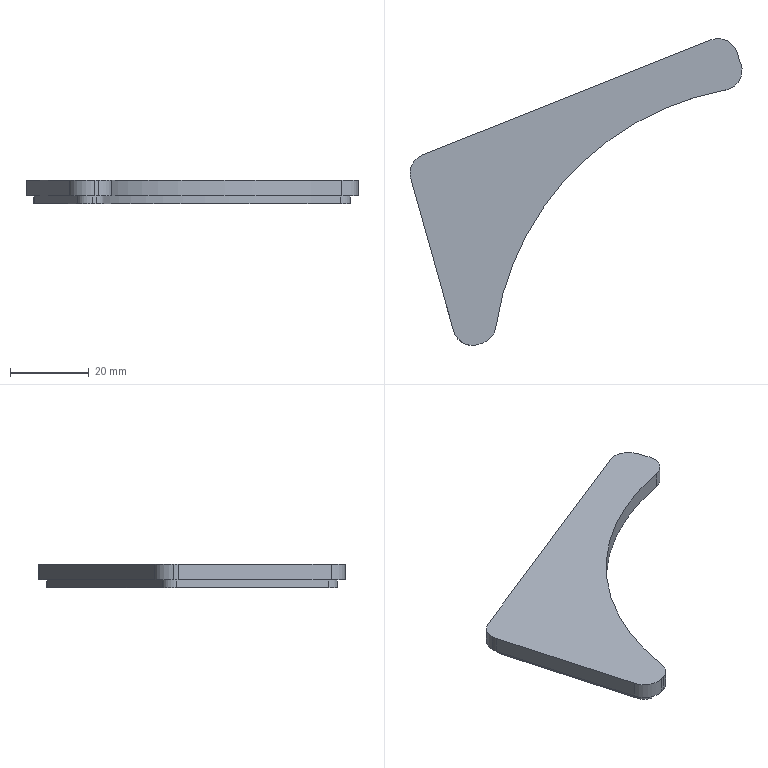Part | SolidWorks | features Extrusion 1, ICE 1 | 1 solid | 25 faces | box 84.083 x 77.703 x 6 mm | volume 11123 mm3 | cylinder 14 | plane 11 | commonest cylinder face diameters 6 x6 10 x6 144 x1 148 x1
STEP:
#1=CARTESIAN_POINT('',(135.377,149.372,4.));
#2=VERTEX_POINT('',#1);
#3=CARTESIAN_POINT('',(135.564,148.019,4.));
#4=VERTEX_POINT('',#3);
#5=CARTESIAN_POINT('',(140.377,149.372,4.));
#6=DIRECTION('',(0.,0.,1.));
#7=DIRECTION('',(-1.,0.,0.));
#8=AXIS2_PLACEMENT_3D('',#5,#6,#7);
#9=CIRCLE('',#8,5.);
#10=EDGE_CURVE('',#2,#4,#9,.T.);
#11=ORIENTED_EDGE('',*,*,#10,.F.);
#12=CARTESIAN_POINT('',(135.377,149.372,0.));
#13=VERTEX_POINT('',#12);
#14=CARTESIAN_POINT('',(135.377,149.372,4.));
#15=DIRECTION('',(0.,0.,-1.));
#16=VECTOR('',#15,1000.);
#17=LINE('',#14,#16);
#18=EDGE_CURVE('',#2,#13,#17,.T.);
#19=ORIENTED_EDGE('',*,*,#18,.T.);
#20=CARTESIAN_POINT('',(135.564,148.019,0.));
#21=VERTEX_POINT('',#20);
#22=CARTESIAN_POINT('',(140.377,149.372,0.));
#23=DIRECTION('',(0.,0.,1.));
#24=DIRECTION('',(-1.,0.,0.));
#25=AXIS2_PLACEMENT_3D('',#22,#23,#24);
#26=CIRCLE('',#25,5.);
#27=EDGE_CURVE('',#13,#21,#26,.T.);
#28=ORIENTED_EDGE('',*,*,#27,.T.);
#29=CARTESIAN_POINT('',(135.564,148.019,4.));
#30=DIRECTION('',(0.,0.,-1.));
#31=VECTOR('',#30,1000.);
#32=LINE('',#29,#31);
#33=EDGE_CURVE('',#4,#21,#32,.T.);
#34=ORIENTED_EDGE('',*,*,#33,.F.);
#35=EDGE_LOOP('',(#11,#19,#28,#34));
#36=FACE_OUTER_BOUND('',#35,.T.);
#37=CARTESIAN_POINT('',(140.377,149.372,4.));
#38=DIRECTION('',(0.,0.,-1.));
#39=DIRECTION('',(-1.,0.,0.));
#40=AXIS2_PLACEMENT_3D('',#37,#38,#39);
#41=CYLINDRICAL_SURFACE('',#40,5.);
#42=ADVANCED_FACE('',(#36),#41,.T.);
#43=CARTESIAN_POINT('',(214.999,172.437,-2.));
#44=VERTEX_POINT('',#43);
#45=CARTESIAN_POINT('',(217.46,175.388,-2.));
#46=VERTEX_POINT('',#45);
#47=CARTESIAN_POINT('',(214.46,175.388,-2.));
#48=DIRECTION('',(0.,0.,1.));
#49=DIRECTION('',(1.,0.,0.));
#50=AXIS2_PLACEMENT_3D('',#47,#48,#49);
#51=CIRCLE('',#50,3.);
#52=EDGE_CURVE('',#44,#46,#51,.T.);
#53=ORIENTED_EDGE('',*,*,#52,.T.);
#54=CARTESIAN_POINT('',(217.46,175.388,0.));
#55=VERTEX_POINT('',#54);
#56=CARTESIAN_POINT('',(217.46,175.388,-2.));
#57=DIRECTION('',(0.,0.,1.));
#58=VECTOR('',#57,1000.);
#59=LINE('',#56,#58);
#60=EDGE_CURVE('',#46,#55,#59,.T.);
#61=ORIENTED_EDGE('',*,*,#60,.T.);
#62=CARTESIAN_POINT('',(214.999,172.437,0.));
#63=VERTEX_POINT('',#62);
#64=CARTESIAN_POINT('',(214.46,175.388,0.));
#65=DIRECTION('',(0.,0.,1.));
#66=DIRECTION('',(1.,0.,0.));
#67=AXIS2_PLACEMENT_3D('',#64,#65,#66);
#68=CIRCLE('',#67,3.);
#69=EDGE_CURVE('',#63,#55,#68,.T.);
#70=ORIENTED_EDGE('',*,*,#69,.F.);
#71=CARTESIAN_POINT('',(214.999,172.437,-2.));
#72=DIRECTION('',(0.,0.,1.));
#73=VECTOR('',#72,1000.);
#74=LINE('',#71,#73);
#75=EDGE_CURVE('',#44,#63,#74,.T.);
#76=ORIENTED_EDGE('',*,*,#75,.F.);
#77=EDGE_LOOP('',(#53,#61,#70,#76));
#78=FACE_OUTER_BOUND('',#77,.T.);
#79=CARTESIAN_POINT('',(214.46,175.388,-2.));
#80=DIRECTION('',(0.,0.,1.));
#81=DIRECTION('',(1.,0.,0.));
#82=AXIS2_PLACEMENT_3D('',#79,#80,#81);
#83=CYLINDRICAL_SURFACE('',#82,3.);
#84=ADVANCED_FACE('',(#78),#83,.T.);
#85=CARTESIAN_POINT('',(139.266,152.159,0.));
#86=VERTEX_POINT('',#85);
#87=CARTESIAN_POINT('',(137.489,148.561,0.));
#88=VERTEX_POINT('',#87);
#89=CARTESIAN_POINT('',(140.377,149.372,0.));
#90=DIRECTION('',(0.,0.,1.));
#91=DIRECTION('',(1.,0.,0.));
#92=AXIS2_PLACEMENT_3D('',#89,#90,#91);
#93=CIRCLE('',#92,3.);
#94=EDGE_CURVE('',#86,#88,#93,.T.);
#95=ORIENTED_EDGE('',*,*,#94,.F.);
#96=CARTESIAN_POINT('',(139.266,152.159,-2.));
#97=VERTEX_POINT('',#96);
#98=CARTESIAN_POINT('',(139.266,152.159,-2.));
#99=DIRECTION('',(0.,0.,1.));
#100=VECTOR('',#99,1000.);
#101=LINE('',#98,#100);
#102=EDGE_CURVE('',#97,#86,#101,.T.);
#103=ORIENTED_EDGE('',*,*,#102,.F.);
#104=CARTESIAN_POINT('',(137.489,148.561,-2.));
#105=VERTEX_POINT('',#104);
#106=CARTESIAN_POINT('',(140.377,149.372,-2.));
#107=DIRECTION('',(0.,0.,1.));
#108=DIRECTION('',(1.,0.,0.));
#109=AXIS2_PLACEMENT_3D('',#106,#107,#108);
#110=CIRCLE('',#109,3.);
#111=EDGE_CURVE('',#97,#105,#110,.T.);
#112=ORIENTED_EDGE('',*,*,#111,.T.);
#113=CARTESIAN_POINT('',(137.489,148.561,-2.));
#114=DIRECTION('',(0.,0.,1.));
#115=VECTOR('',#114,1000.);
#116=LINE('',#113,#115);
#117=EDGE_CURVE('',#105,#88,#116,.T.);
#118=ORIENTED_EDGE('',*,*,#117,.T.);
#119=EDGE_LOOP('',(#95,#103,#112,#118));
#120=FACE_OUTER_BOUND('',#119,.T.);
#121=CARTESIAN_POINT('',(140.377,149.372,-2.));
#122=DIRECTION('',(0.,0.,1.));
#123=DIRECTION('',(1.,0.,0.));
#124=AXIS2_PLACEMENT_3D('',#121,#122,#123);
#125=CYLINDRICAL_SURFACE('',#124,3.);
#126=ADVANCED_FACE('',(#120),#125,.T.);
#127=CARTESIAN_POINT('',(212.285,181.276,0.));
#128=VERTEX_POINT('',#127);
#129=CARTESIAN_POINT('',(212.285,181.276,0.));
#130=DIRECTION('',(-0.9289,-0.3704,0.));
#131=VECTOR('',#130,1000.);
#132=LINE('',#129,#131);
#133=EDGE_CURVE('',#128,#86,#132,.T.);
#134=ORIENTED_EDGE('',*,*,#133,.F.);
#135=CARTESIAN_POINT('',(212.285,181.276,-2.));
#136=VERTEX_POINT('',#135);
#137=CARTESIAN_POINT('',(212.285,181.276,-2.));
#138=DIRECTION('',(0.,0.,1.));
#139=VECTOR('',#138,1000.);
#140=LINE('',#137,#139);
#141=EDGE_CURVE('',#136,#128,#140,.T.);
#142=ORIENTED_EDGE('',*,*,#141,.F.);
#143=CARTESIAN_POINT('',(212.285,181.276,-2.));
#144=DIRECTION('',(-0.9289,-0.3704,0.));
#145=VECTOR('',#144,1000.);
#146=LINE('',#143,#145);
#147=EDGE_CURVE('',#136,#97,#146,.T.);
#148=ORIENTED_EDGE('',*,*,#147,.T.);
#149=ORIENTED_EDGE('',*,*,#102,.T.);
#150=EDGE_LOOP('',(#134,#142,#148,#149));
#151=FACE_OUTER_BOUND('',#150,.T.);
#152=CARTESIAN_POINT('',(212.285,181.276,-2.));
#153=DIRECTION('',(-0.3704,0.9289,0.));
#154=DIRECTION('',(-0.9289,-0.3704,0.));
#155=AXIS2_PLACEMENT_3D('',#152,#153,#154);
#156=PLANE('',#155);
#157=ADVANCED_FACE('',(#151),#156,.T.);
#158=CARTESIAN_POINT('',(216.234,179.463,0.));
#159=VERTEX_POINT('',#158);
#160=CARTESIAN_POINT('',(213.396,178.489,0.));
#161=DIRECTION('',(0.,0.,1.));
#162=DIRECTION('',(1.,0.,0.));
#163=AXIS2_PLACEMENT_3D('',#160,#161,#162);
#164=CIRCLE('',#163,3.);
#165=EDGE_CURVE('',#159,#128,#164,.T.);
#166=ORIENTED_EDGE('',*,*,#165,.F.);
#167=CARTESIAN_POINT('',(216.234,179.463,-2.));
#168=VERTEX_POINT('',#167);
#169=CARTESIAN_POINT('',(216.234,179.463,-2.));
#170=DIRECTION('',(0.,0.,1.));
#171=VECTOR('',#170,1000.);
#172=LINE('',#169,#171);
#173=EDGE_CURVE('',#168,#159,#172,.T.);
#174=ORIENTED_EDGE('',*,*,#173,.F.);
#175=CARTESIAN_POINT('',(213.396,178.489,-2.));
#176=DIRECTION('',(0.,0.,1.));
#177=DIRECTION('',(1.,0.,0.));
#178=AXIS2_PLACEMENT_3D('',#175,#176,#177);
#179=CIRCLE('',#178,3.);
#180=EDGE_CURVE('',#168,#136,#179,.T.);
#181=ORIENTED_EDGE('',*,*,#180,.T.);
#182=ORIENTED_EDGE('',*,*,#141,.T.);
#183=EDGE_LOOP('',(#166,#174,#181,#182));
#184=FACE_OUTER_BOUND('',#183,.T.);
#185=CARTESIAN_POINT('',(213.396,178.489,-2.));
#186=DIRECTION('',(0.,0.,1.));
#187=DIRECTION('',(1.,0.,0.));
#188=AXIS2_PLACEMENT_3D('',#185,#186,#187);
#189=CYLINDRICAL_SURFACE('',#188,3.);
#190=ADVANCED_FACE('',(#184),#189,.T.);
#191=CARTESIAN_POINT('',(217.298,176.361,0.));
#192=VERTEX_POINT('',#191);
#193=CARTESIAN_POINT('',(217.298,176.361,0.));
#194=DIRECTION('',(-0.3245,0.9459,0.));
#195=VECTOR('',#194,1000.);
#196=LINE('',#193,#195);
#197=EDGE_CURVE('',#192,#159,#196,.T.);
#198=ORIENTED_EDGE('',*,*,#197,.F.);
#199=CARTESIAN_POINT('',(217.298,176.361,-2.));
#200=VERTEX_POINT('',#199);
#201=CARTESIAN_POINT('',(217.298,176.361,-2.));
#202=DIRECTION('',(0.,0.,1.));
#203=VECTOR('',#202,1000.);
#204=LINE('',#201,#203);
#205=EDGE_CURVE('',#200,#192,#204,.T.);
#206=ORIENTED_EDGE('',*,*,#205,.F.);
#207=CARTESIAN_POINT('',(217.298,176.361,-2.));
#208=DIRECTION('',(-0.3245,0.9459,0.));
#209=VECTOR('',#208,1000.);
#210=LINE('',#207,#209);
#211=EDGE_CURVE('',#200,#168,#210,.T.);
#212=ORIENTED_EDGE('',*,*,#211,.T.);
#213=ORIENTED_EDGE('',*,*,#173,.T.);
#214=EDGE_LOOP('',(#198,#206,#212,#213));
#215=FACE_OUTER_BOUND('',#214,.T.);
#216=CARTESIAN_POINT('',(217.298,176.361,-2.));
#217=DIRECTION('',(0.9459,0.3245,0.));
#218=DIRECTION('',(-0.3245,0.9459,0.));
#219=AXIS2_PLACEMENT_3D('',#216,#217,#218);
#220=PLANE('',#219);
#221=ADVANCED_FACE('',(#215),#220,.T.);
#222=ORIENTED_EDGE('',*,*,#60,.F.);
#223=CARTESIAN_POINT('',(214.46,175.388,-2.));
#224=DIRECTION('',(0.,0.,1.));
#225=DIRECTION('',(1.,0.,0.));
#226=AXIS2_PLACEMENT_3D('',#223,#224,#225);
#227=CIRCLE('',#226,3.);
#228=EDGE_CURVE('',#46,#200,#227,.T.);
#229=ORIENTED_EDGE('',*,*,#228,.T.);
#230=ORIENTED_EDGE('',*,*,#205,.T.);
#231=CARTESIAN_POINT('',(214.46,175.388,0.));
#232=DIRECTION('',(0.,0.,1.));
#233=DIRECTION('',(1.,0.,0.));
#234=AXIS2_PLACEMENT_3D('',#231,#232,#233);
#235=CIRCLE('',#234,3.);
#236=EDGE_CURVE('',#55,#192,#235,.T.);
#237=ORIENTED_EDGE('',*,*,#236,.F.);
#238=EDGE_LOOP('',(#222,#229,#230,#237));
#239=FACE_OUTER_BOUND('',#238,.T.);
#240=CARTESIAN_POINT('',(214.46,175.388,-2.));
#241=DIRECTION('',(0.,0.,1.));
#242=DIRECTION('',(1.,0.,0.));
#243=AXIS2_PLACEMENT_3D('',#240,#241,#242);
#244=CYLINDRICAL_SURFACE('',#243,3.);
#245=ADVANCED_FACE('',(#239),#244,.T.);
#246=CARTESIAN_POINT('',(155.118,110.657,0.));
#247=VERTEX_POINT('',#246);
#248=CARTESIAN_POINT('',(228.293,99.641,0.));
#249=DIRECTION('',(0.,0.,-1.));
#250=DIRECTION('',(1.,0.,0.));
#251=AXIS2_PLACEMENT_3D('',#248,#249,#250);
#252=CIRCLE('',#251,74.);
#253=EDGE_CURVE('',#247,#63,#252,.T.);
#254=ORIENTED_EDGE('',*,*,#253,.F.);
#255=CARTESIAN_POINT('',(155.118,110.657,-2.));
#256=VERTEX_POINT('',#255);
#257=CARTESIAN_POINT('',(155.118,110.657,-2.));
#258=DIRECTION('',(0.,0.,1.));
#259=VECTOR('',#258,1000.);
#260=LINE('',#257,#259);
#261=EDGE_CURVE('',#256,#247,#260,.T.);
#262=ORIENTED_EDGE('',*,*,#261,.F.);
#263=CARTESIAN_POINT('',(228.293,99.641,-2.));
#264=DIRECTION('',(0.,0.,-1.));
#265=DIRECTION('',(1.,0.,0.));
#266=AXIS2_PLACEMENT_3D('',#263,#264,#265);
#267=CIRCLE('',#266,74.);
#268=EDGE_CURVE('',#256,#44,#267,.T.);
#269=ORIENTED_EDGE('',*,*,#268,.T.);
#270=ORIENTED_EDGE('',*,*,#75,.T.);
#271=EDGE_LOOP('',(#254,#262,#269,#270));
#272=FACE_OUTER_BOUND('',#271,.T.);
#273=CARTESIAN_POINT('',(228.293,99.641,-2.));
#274=DIRECTION('',(0.,0.,1.));
#275=DIRECTION('',(1.,0.,0.));
#276=AXIS2_PLACEMENT_3D('',#273,#274,#275);
#277=CYLINDRICAL_SURFACE('',#276,74.);
#278=ADVANCED_FACE('',(#272),#277,.F.);
#279=CARTESIAN_POINT('',(153.125,108.266,0.));
#280=VERTEX_POINT('',#279);
#281=CARTESIAN_POINT('',(152.151,111.104,0.));
#282=DIRECTION('',(0.,0.,1.));
#283=DIRECTION('',(1.,0.,0.));
#284=AXIS2_PLACEMENT_3D('',#281,#282,#283);
#285=CIRCLE('',#284,3.);
#286=EDGE_CURVE('',#280,#247,#285,.T.);
#287=ORIENTED_EDGE('',*,*,#286,.F.);
#288=CARTESIAN_POINT('',(153.125,108.266,-2.));
#289=VERTEX_POINT('',#288);
#290=CARTESIAN_POINT('',(153.125,108.266,-2.));
#291=DIRECTION('',(0.,0.,1.));
#292=VECTOR('',#291,1000.);
#293=LINE('',#290,#292);
#294=EDGE_CURVE('',#289,#280,#293,.T.);
#295=ORIENTED_EDGE('',*,*,#294,.F.);
#296=CARTESIAN_POINT('',(152.151,111.104,-2.));
#297=DIRECTION('',(0.,0.,1.));
#298=DIRECTION('',(1.,0.,0.));
#299=AXIS2_PLACEMENT_3D('',#296,#297,#298);
#300=CIRCLE('',#299,3.);
#301=EDGE_CURVE('',#289,#256,#300,.T.);
#302=ORIENTED_EDGE('',*,*,#301,.T.);
#303=ORIENTED_EDGE('',*,*,#261,.T.);
#304=EDGE_LOOP('',(#287,#295,#302,#303));
#305=FACE_OUTER_BOUND('',#304,.T.);
#306=CARTESIAN_POINT('',(152.151,111.104,-2.));
#307=DIRECTION('',(0.,0.,1.));
#308=DIRECTION('',(1.,0.,0.));
#309=AXIS2_PLACEMENT_3D('',#306,#307,#308);
#310=CYLINDRICAL_SURFACE('',#309,3.);
#311=ADVANCED_FACE('',(#305),#310,.T.);
#312=CARTESIAN_POINT('',(152.197,107.948,0.));
#313=VERTEX_POINT('',#312);
#314=CARTESIAN_POINT('',(152.197,107.948,0.));
#315=DIRECTION('',(0.9459,0.3245,0.));
#316=VECTOR('',#315,1000.);
#317=LINE('',#314,#316);
#318=EDGE_CURVE('',#313,#280,#317,.T.);
#319=ORIENTED_EDGE('',*,*,#318,.F.);
#320=CARTESIAN_POINT('',(152.197,107.948,-2.));
#321=VERTEX_POINT('',#320);
#322=CARTESIAN_POINT('',(152.197,107.948,-2.));
#323=DIRECTION('',(0.,0.,1.));
#324=VECTOR('',#323,1000.);
#325=LINE('',#322,#324);
#326=EDGE_CURVE('',#321,#313,#325,.T.);
#327=ORIENTED_EDGE('',*,*,#326,.F.);
#328=CARTESIAN_POINT('',(152.197,107.948,-2.));
#329=DIRECTION('',(0.9459,0.3245,0.));
#330=VECTOR('',#329,1000.);
#331=LINE('',#328,#330);
#332=EDGE_CURVE('',#321,#289,#331,.T.);
#333=ORIENTED_EDGE('',*,*,#332,.T.);
#334=ORIENTED_EDGE('',*,*,#294,.T.);
#335=EDGE_LOOP('',(#319,#327,#333,#334));
#336=FACE_OUTER_BOUND('',#335,.T.);
#337=CARTESIAN_POINT('',(152.197,107.948,-2.));
#338=DIRECTION('',(0.3245,-0.9459,0.));
#339=DIRECTION('',(0.9459,0.3245,0.));
#340=AXIS2_PLACEMENT_3D('',#337,#338,#339);
#341=PLANE('',#340);
#342=ADVANCED_FACE('',(#336),#341,.T.);
#343=CARTESIAN_POINT('',(148.336,109.974,0.));
#344=VERTEX_POINT('',#343);
#345=CARTESIAN_POINT('',(151.224,110.786,0.));
#346=DIRECTION('',(0.,0.,1.));
#347=DIRECTION('',(1.,0.,0.));
#348=AXIS2_PLACEMENT_3D('',#345,#346,#347);
#349=CIRCLE('',#348,3.);
#350=EDGE_CURVE('',#344,#313,#349,.T.);
#351=ORIENTED_EDGE('',*,*,#350,.F.);
#352=CARTESIAN_POINT('',(148.336,109.974,-2.));
#353=VERTEX_POINT('',#352);
#354=CARTESIAN_POINT('',(148.336,109.974,-2.));
#355=DIRECTION('',(0.,0.,1.));
#356=VECTOR('',#355,1000.);
#357=LINE('',#354,#356);
#358=EDGE_CURVE('',#353,#344,#357,.T.);
#359=ORIENTED_EDGE('',*,*,#358,.F.);
#360=CARTESIAN_POINT('',(151.224,110.786,-2.));
#361=DIRECTION('',(0.,0.,1.));
#362=DIRECTION('',(1.,0.,0.));
#363=AXIS2_PLACEMENT_3D('',#360,#361,#362);
#364=CIRCLE('',#363,3.);
#365=EDGE_CURVE('',#353,#321,#364,.T.);
#366=ORIENTED_EDGE('',*,*,#365,.T.);
#367=ORIENTED_EDGE('',*,*,#326,.T.);
#368=EDGE_LOOP('',(#351,#359,#366,#367));
#369=FACE_OUTER_BOUND('',#368,.T.);
#370=CARTESIAN_POINT('',(151.224,110.786,-2.));
#371=DIRECTION('',(0.,0.,1.));
#372=DIRECTION('',(1.,0.,0.));
#373=AXIS2_PLACEMENT_3D('',#370,#371,#372);
#374=CYLINDRICAL_SURFACE('',#373,3.);
#375=ADVANCED_FACE('',(#369),#374,.T.);
#376=CARTESIAN_POINT('',(137.489,148.561,0.));
#377=DIRECTION('',(0.2706,-0.9627,0.));
#378=VECTOR('',#377,1000.);
#379=LINE('',#376,#378);
#380=EDGE_CURVE('',#88,#344,#379,.T.);
#381=ORIENTED_EDGE('',*,*,#380,.F.);
#382=ORIENTED_EDGE('',*,*,#117,.F.);
#383=CARTESIAN_POINT('',(137.489,148.561,-2.));
#384=DIRECTION('',(0.2706,-0.9627,0.));
#385=VECTOR('',#384,1000.);
#386=LINE('',#383,#385);
#387=EDGE_CURVE('',#105,#353,#386,.T.);
#388=ORIENTED_EDGE('',*,*,#387,.T.);
#389=ORIENTED_EDGE('',*,*,#358,.T.);
#390=EDGE_LOOP('',(#381,#382,#388,#389));
#391=FACE_OUTER_BOUND('',#390,.T.);
#392=CARTESIAN_POINT('',(137.489,148.561,-2.));
#393=DIRECTION('',(-0.9627,-0.2706,0.));
#394=DIRECTION('',(0.2706,-0.9627,0.));
#395=AXIS2_PLACEMENT_3D('',#392,#393,#394);
#396=PLANE('',#395);
#397=ADVANCED_FACE('',(#391),#396,.T.);
#398=ORIENTED_EDGE('',*,*,#111,.F.);
#399=ORIENTED_EDGE('',*,*,#147,.F.);
#400=ORIENTED_EDGE('',*,*,#180,.F.);
#401=ORIENTED_EDGE('',*,*,#211,.F.);
#402=ORIENTED_EDGE('',*,*,#228,.F.);
#403=ORIENTED_EDGE('',*,*,#52,.F.);
#404=ORIENTED_EDGE('',*,*,#268,.F.);
#405=ORIENTED_EDGE('',*,*,#301,.F.);
#406=ORIENTED_EDGE('',*,*,#332,.F.);
#407=ORIENTED_EDGE('',*,*,#365,.F.);
#408=ORIENTED_EDGE('',*,*,#387,.F.);
#409=EDGE_LOOP('',(#398,#399,#400,#401,#402,#403,#404,#405,#406,#407,#408));
#410=FACE_OUTER_BOUND('',#409,.T.);
#411=CARTESIAN_POINT('',(140.377,149.372,-2.));
#412=DIRECTION('',(0.,0.,1.));
#413=DIRECTION('',(1.,0.,0.));
#414=AXIS2_PLACEMENT_3D('',#411,#412,#413);
#415=PLANE('',#414);
#416=ADVANCED_FACE('',(#410),#415,.F.);
#417=CARTESIAN_POINT('',(153.774,106.374,0.));
#418=VERTEX_POINT('',#417);
#419=CARTESIAN_POINT('',(157.095,110.359,0.));
#420=VERTEX_POINT('',#419);
#421=CARTESIAN_POINT('',(152.151,111.104,0.));
#422=DIRECTION('',(0.,0.,1.));
#423=DIRECTION('',(-1.,0.,0.));
#424=AXIS2_PLACEMENT_3D('',#421,#422,#423);
#425=CIRCLE('',#424,5.);
#426=EDGE_CURVE('',#418,#420,#425,.T.);
#427=ORIENTED_EDGE('',*,*,#426,.T.);
#428=CARTESIAN_POINT('',(157.095,110.359,4.));
#429=VERTEX_POINT('',#428);
#430=CARTESIAN_POINT('',(157.095,110.359,4.));
#431=DIRECTION('',(0.,0.,-1.));
#432=VECTOR('',#431,1000.);
#433=LINE('',#430,#432);
#434=EDGE_CURVE('',#429,#420,#433,.T.);
#435=ORIENTED_EDGE('',*,*,#434,.F.);
#436=CARTESIAN_POINT('',(153.774,106.374,4.));
#437=VERTEX_POINT('',#436);
#438=CARTESIAN_POINT('',(152.151,111.104,4.));
#439=DIRECTION('',(0.,0.,1.));
#440=DIRECTION('',(-1.,0.,0.));
#441=AXIS2_PLACEMENT_3D('',#438,#439,#440);
#442=CIRCLE('',#441,5.);
#443=EDGE_CURVE('',#437,#429,#442,.T.);
#444=ORIENTED_EDGE('',*,*,#443,.F.);
#445=CARTESIAN_POINT('',(153.774,106.374,4.));
#446=DIRECTION('',(0.,0.,-1.));
#447=VECTOR('',#446,1000.);
#448=LINE('',#445,#447);
#449=EDGE_CURVE('',#437,#418,#448,.T.);
#450=ORIENTED_EDGE('',*,*,#449,.T.);
#451=EDGE_LOOP('',(#427,#435,#444,#450));
#452=FACE_OUTER_BOUND('',#451,.T.);
#453=CARTESIAN_POINT('',(152.151,111.104,4.));
#454=DIRECTION('',(0.,0.,-1.));
#455=DIRECTION('',(-1.,0.,0.));
#456=AXIS2_PLACEMENT_3D('',#453,#454,#455);
#457=CYLINDRICAL_SURFACE('',#456,5.);
#458=ADVANCED_FACE('',(#452),#457,.T.);
#459=CARTESIAN_POINT('',(215.358,170.469,0.));
#460=VERTEX_POINT('',#459);
#461=CARTESIAN_POINT('',(228.293,99.641,0.));
#462=DIRECTION('',(0.,0.,-1.));
#463=DIRECTION('',(-1.,0.,0.));
#464=AXIS2_PLACEMENT_3D('',#461,#462,#463);
#465=CIRCLE('',#464,72.);
#466=EDGE_CURVE('',#420,#460,#465,.T.);
#467=ORIENTED_EDGE('',*,*,#466,.T.);
#468=CARTESIAN_POINT('',(215.358,170.469,4.));
#469=VERTEX_POINT('',#468);
#470=CARTESIAN_POINT('',(215.358,170.469,4.));
#471=DIRECTION('',(0.,0.,-1.));
#472=VECTOR('',#471,1000.);
#473=LINE('',#470,#472);
#474=EDGE_CURVE('',#469,#460,#473,.T.);
#475=ORIENTED_EDGE('',*,*,#474,.F.);
#476=CARTESIAN_POINT('',(228.293,99.641,4.));
#477=DIRECTION('',(0.,0.,-1.));
#478=DIRECTION('',(-1.,0.,0.));
#479=AXIS2_PLACEMENT_3D('',#476,#477,#478);
#480=CIRCLE('',#479,72.);
#481=EDGE_CURVE('',#429,#469,#480,.T.);
#482=ORIENTED_EDGE('',*,*,#481,.F.);
#483=ORIENTED_EDGE('',*,*,#434,.T.);
#484=EDGE_LOOP('',(#467,#475,#482,#483));
#485=FACE_OUTER_BOUND('',#484,.T.);
#486=CARTESIAN_POINT('',(228.293,99.641,4.));
#487=DIRECTION('',(0.,0.,-1.));
#488=DIRECTION('',(-1.,0.,0.));
#489=AXIS2_PLACEMENT_3D('',#486,#487,#488);
#490=CYLINDRICAL_SURFACE('',#489,72.);
#491=ADVANCED_FACE('',(#485),#490,.F.);
#492=CARTESIAN_POINT('',(219.189,177.01,0.));
#493=VERTEX_POINT('',#492);
#494=CARTESIAN_POINT('',(214.46,175.388,0.));
#495=DIRECTION('',(0.,0.,1.));
#496=DIRECTION('',(-1.,0.,0.));
#497=AXIS2_PLACEMENT_3D('',#494,#495,#496);
#498=CIRCLE('',#497,5.);
#499=EDGE_CURVE('',#460,#493,#498,.T.);
#500=ORIENTED_EDGE('',*,*,#499,.T.);
#501=CARTESIAN_POINT('',(219.189,177.01,4.));
#502=VERTEX_POINT('',#501);
#503=CARTESIAN_POINT('',(219.189,177.01,4.));
#504=DIRECTION('',(0.,0.,-1.));
#505=VECTOR('',#504,1000.);
#506=LINE('',#503,#505);
#507=EDGE_CURVE('',#502,#493,#506,.T.);
#508=ORIENTED_EDGE('',*,*,#507,.F.);
#509=CARTESIAN_POINT('',(214.46,175.388,4.));
#510=DIRECTION('',(0.,0.,1.));
#511=DIRECTION('',(-1.,0.,0.));
#512=AXIS2_PLACEMENT_3D('',#509,#510,#511);
#513=CIRCLE('',#512,5.);
#514=EDGE_CURVE('',#469,#502,#513,.T.);
#515=ORIENTED_EDGE('',*,*,#514,.F.);
#516=ORIENTED_EDGE('',*,*,#474,.T.);
#517=EDGE_LOOP('',(#500,#508,#515,#516));
#518=FACE_OUTER_BOUND('',#517,.T.);
#519=CARTESIAN_POINT('',(214.46,175.388,4.));
#520=DIRECTION('',(0.,0.,-1.));
#521=DIRECTION('',(-1.,0.,0.));
#522=AXIS2_PLACEMENT_3D('',#519,#520,#521);
#523=CYLINDRICAL_SURFACE('',#522,5.);
#524=ADVANCED_FACE('',(#518),#523,.T.);
#525=CARTESIAN_POINT('',(218.125,180.112,0.));
#526=VERTEX_POINT('',#525);
#527=CARTESIAN_POINT('',(218.125,180.112,0.));
#528=DIRECTION('',(-0.3245,0.9459,0.));
#529=VECTOR('',#528,1000.);
#530=LINE('',#527,#529);
#531=EDGE_CURVE('',#493,#526,#530,.T.);
#532=ORIENTED_EDGE('',*,*,#531,.T.);
#533=CARTESIAN_POINT('',(218.125,180.112,4.));
#534=VERTEX_POINT('',#533);
#535=CARTESIAN_POINT('',(218.125,180.112,4.));
#536=DIRECTION('',(0.,0.,-1.));
#537=VECTOR('',#536,1000.);
#538=LINE('',#535,#537);
#539=EDGE_CURVE('',#534,#526,#538,.T.);
#540=ORIENTED_EDGE('',*,*,#539,.F.);
#541=CARTESIAN_POINT('',(218.125,180.112,4.));
#542=DIRECTION('',(-0.3245,0.9459,0.));
#543=VECTOR('',#542,1000.);
#544=LINE('',#541,#543);
#545=EDGE_CURVE('',#502,#534,#544,.T.);
#546=ORIENTED_EDGE('',*,*,#545,.F.);
#547=ORIENTED_EDGE('',*,*,#507,.T.);
#548=EDGE_LOOP('',(#532,#540,#546,#547));
#549=FACE_OUTER_BOUND('',#548,.T.);
#550=CARTESIAN_POINT('',(218.125,180.112,4.));
#551=DIRECTION('',(-0.9459,-0.3245,0.));
#552=DIRECTION('',(0.3245,-0.9459,0.));
#553=AXIS2_PLACEMENT_3D('',#550,#551,#552);
#554=PLANE('',#553);
#555=ADVANCED_FACE('',(#549),#554,.F.);
#556=CARTESIAN_POINT('',(211.544,183.134,0.));
#557=VERTEX_POINT('',#556);
#558=CARTESIAN_POINT('',(213.396,178.489,0.));
#559=DIRECTION('',(0.,0.,1.));
#560=DIRECTION('',(-1.,0.,0.));
#561=AXIS2_PLACEMENT_3D('',#558,#559,#560);
#562=CIRCLE('',#561,5.);
#563=EDGE_CURVE('',#526,#557,#562,.T.);
#564=ORIENTED_EDGE('',*,*,#563,.T.);
#565=CARTESIAN_POINT('',(211.544,183.134,4.));
#566=VERTEX_POINT('',#565);
#567=CARTESIAN_POINT('',(211.544,183.134,4.));
#568=DIRECTION('',(0.,0.,-1.));
#569=VECTOR('',#568,1000.);
#570=LINE('',#567,#569);
#571=EDGE_CURVE('',#566,#557,#570,.T.);
#572=ORIENTED_EDGE('',*,*,#571,.F.);
#573=CARTESIAN_POINT('',(213.396,178.489,4.));
#574=DIRECTION('',(0.,0.,1.));
#575=DIRECTION('',(-1.,0.,0.));
#576=AXIS2_PLACEMENT_3D('',#573,#574,#575);
#577=CIRCLE('',#576,5.);
#578=EDGE_CURVE('',#534,#566,#577,.T.);
#579=ORIENTED_EDGE('',*,*,#578,.F.);
#580=ORIENTED_EDGE('',*,*,#539,.T.);
#581=EDGE_LOOP('',(#564,#572,#579,#580));
#582=FACE_OUTER_BOUND('',#581,.T.);
#583=CARTESIAN_POINT('',(213.396,178.489,4.));
#584=DIRECTION('',(0.,0.,-1.));
#585=DIRECTION('',(-1.,0.,0.));
#586=AXIS2_PLACEMENT_3D('',#583,#584,#585);
#587=CYLINDRICAL_SURFACE('',#586,5.);
#588=ADVANCED_FACE('',(#582),#587,.T.);
#589=CARTESIAN_POINT('',(138.525,154.017,0.));
#590=VERTEX_POINT('',#589);
#591=CARTESIAN_POINT('',(138.525,154.017,0.));
#592=DIRECTION('',(-0.9289,-0.3704,0.));
#593=VECTOR('',#592,1000.);
#594=LINE('',#591,#593);
#595=EDGE_CURVE('',#557,#590,#594,.T.);
#596=ORIENTED_EDGE('',*,*,#595,.T.);
#597=CARTESIAN_POINT('',(138.525,154.017,4.));
#598=VERTEX_POINT('',#597);
#599=CARTESIAN_POINT('',(138.525,154.017,4.));
#600=DIRECTION('',(0.,0.,-1.));
#601=VECTOR('',#600,1000.);
#602=LINE('',#599,#601);
#603=EDGE_CURVE('',#598,#590,#602,.T.);
#604=ORIENTED_EDGE('',*,*,#603,.F.);
#605=CARTESIAN_POINT('',(138.525,154.017,4.));
#606=DIRECTION('',(-0.9289,-0.3704,0.));
#607=VECTOR('',#606,1000.);
#608=LINE('',#605,#607);
#609=EDGE_CURVE('',#566,#598,#608,.T.);
#610=ORIENTED_EDGE('',*,*,#609,.F.);
#611=ORIENTED_EDGE('',*,*,#571,.T.);
#612=EDGE_LOOP('',(#596,#604,#610,#611));
#613=FACE_OUTER_BOUND('',#612,.T.);
#614=CARTESIAN_POINT('',(138.525,154.017,4.));
#615=DIRECTION('',(0.3704,-0.9289,0.));
#616=DIRECTION('',(0.9289,0.3704,0.));
#617=AXIS2_PLACEMENT_3D('',#614,#615,#616);
#618=PLANE('',#617);
#619=ADVANCED_FACE('',(#613),#618,.F.);
#620=ORIENTED_EDGE('',*,*,#18,.F.);
#621=CARTESIAN_POINT('',(140.377,149.372,4.));
#622=DIRECTION('',(0.,0.,1.));
#623=DIRECTION('',(-1.,0.,0.));
#624=AXIS2_PLACEMENT_3D('',#621,#622,#623);
#625=CIRCLE('',#624,5.);
#626=EDGE_CURVE('',#598,#2,#625,.T.);
#627=ORIENTED_EDGE('',*,*,#626,.F.);
#628=ORIENTED_EDGE('',*,*,#603,.T.);
#629=CARTESIAN_POINT('',(140.377,149.372,0.));
#630=DIRECTION('',(0.,0.,1.));
#631=DIRECTION('',(-1.,0.,0.));
#632=AXIS2_PLACEMENT_3D('',#629,#630,#631);
#633=CIRCLE('',#632,5.);
#634=EDGE_CURVE('',#590,#13,#633,.T.);
#635=ORIENTED_EDGE('',*,*,#634,.T.);
#636=EDGE_LOOP('',(#620,#627,#628,#635));
#637=FACE_OUTER_BOUND('',#636,.T.);
#638=CARTESIAN_POINT('',(140.377,149.372,4.));
#639=DIRECTION('',(0.,0.,-1.));
#640=DIRECTION('',(-1.,0.,0.));
#641=AXIS2_PLACEMENT_3D('',#638,#639,#640);
#642=CYLINDRICAL_SURFACE('',#641,5.);
#643=ADVANCED_FACE('',(#637),#642,.T.);
#644=CARTESIAN_POINT('',(146.41,109.433,0.));
#645=VERTEX_POINT('',#644);
#646=CARTESIAN_POINT('',(146.41,109.433,0.));
#647=DIRECTION('',(0.2706,-0.9627,0.));
#648=VECTOR('',#647,1000.);
#649=LINE('',#646,#648);
#650=EDGE_CURVE('',#21,#645,#649,.T.);
#651=ORIENTED_EDGE('',*,*,#650,.T.);
#652=CARTESIAN_POINT('',(146.41,109.433,4.));
#653=VERTEX_POINT('',#652);
#654=CARTESIAN_POINT('',(146.41,109.433,4.));
#655=DIRECTION('',(0.,0.,-1.));
#656=VECTOR('',#655,1000.);
#657=LINE('',#654,#656);
#658=EDGE_CURVE('',#653,#645,#657,.T.);
#659=ORIENTED_EDGE('',*,*,#658,.F.);
#660=CARTESIAN_POINT('',(146.41,109.433,4.));
#661=DIRECTION('',(0.2706,-0.9627,0.));
#662=VECTOR('',#661,1000.);
#663=LINE('',#660,#662);
#664=EDGE_CURVE('',#4,#653,#663,.T.);
#665=ORIENTED_EDGE('',*,*,#664,.F.);
#666=ORIENTED_EDGE('',*,*,#33,.T.);
#667=EDGE_LOOP('',(#651,#659,#665,#666));
#668=FACE_OUTER_BOUND('',#667,.T.);
#669=CARTESIAN_POINT('',(146.41,109.433,4.));
#670=DIRECTION('',(0.9627,0.2706,0.));
#671=DIRECTION('',(-0.2706,0.9627,0.));
#672=AXIS2_PLACEMENT_3D('',#669,#670,#671);
#673=PLANE('',#672);
#674=ADVANCED_FACE('',(#668),#673,.F.);
#675=CARTESIAN_POINT('',(152.846,106.056,0.));
#676=VERTEX_POINT('',#675);
#677=CARTESIAN_POINT('',(151.224,110.786,0.));
#678=DIRECTION('',(0.,0.,1.));
#679=DIRECTION('',(-1.,0.,0.));
#680=AXIS2_PLACEMENT_3D('',#677,#678,#679);
#681=CIRCLE('',#680,5.);
#682=EDGE_CURVE('',#645,#676,#681,.T.);
#683=ORIENTED_EDGE('',*,*,#682,.T.);
#684=CARTESIAN_POINT('',(152.846,106.056,4.));
#685=VERTEX_POINT('',#684);
#686=CARTESIAN_POINT('',(152.846,106.056,4.));
#687=DIRECTION('',(0.,0.,-1.));
#688=VECTOR('',#687,1000.);
#689=LINE('',#686,#688);
#690=EDGE_CURVE('',#685,#676,#689,.T.);
#691=ORIENTED_EDGE('',*,*,#690,.F.);
#692=CARTESIAN_POINT('',(151.224,110.786,4.));
#693=DIRECTION('',(0.,0.,1.));
#694=DIRECTION('',(-1.,0.,0.));
#695=AXIS2_PLACEMENT_3D('',#692,#693,#694);
#696=CIRCLE('',#695,5.);
#697=EDGE_CURVE('',#653,#685,#696,.T.);
#698=ORIENTED_EDGE('',*,*,#697,.F.);
#699=ORIENTED_EDGE('',*,*,#658,.T.);
#700=EDGE_LOOP('',(#683,#691,#698,#699));
#701=FACE_OUTER_BOUND('',#700,.T.);
#702=CARTESIAN_POINT('',(151.224,110.786,4.));
#703=DIRECTION('',(0.,0.,-1.));
#704=DIRECTION('',(-1.,0.,0.));
#705=AXIS2_PLACEMENT_3D('',#702,#703,#704);
#706=CYLINDRICAL_SURFACE('',#705,5.);
#707=ADVANCED_FACE('',(#701),#706,.T.);
#708=CARTESIAN_POINT('',(153.774,106.374,0.));
#709=DIRECTION('',(0.9459,0.3245,0.));
#710=VECTOR('',#709,1000.);
#711=LINE('',#708,#710);
#712=EDGE_CURVE('',#676,#418,#711,.T.);
#713=ORIENTED_EDGE('',*,*,#712,.T.);
#714=ORIENTED_EDGE('',*,*,#449,.F.);
#715=CARTESIAN_POINT('',(153.774,106.374,4.));
#716=DIRECTION('',(0.9459,0.3245,0.));
#717=VECTOR('',#716,1000.);
#718=LINE('',#715,#717);
#719=EDGE_CURVE('',#685,#437,#718,.T.);
#720=ORIENTED_EDGE('',*,*,#719,.F.);
#721=ORIENTED_EDGE('',*,*,#690,.T.);
#722=EDGE_LOOP('',(#713,#714,#720,#721));
#723=FACE_OUTER_BOUND('',#722,.T.);
#724=CARTESIAN_POINT('',(153.774,106.374,4.));
#725=DIRECTION('',(-0.3245,0.9459,0.));
#726=DIRECTION('',(-0.9459,-0.3245,0.));
#727=AXIS2_PLACEMENT_3D('',#724,#725,#726);
#728=PLANE('',#727);
#729=ADVANCED_FACE('',(#723),#728,.F.);
#730=ORIENTED_EDGE('',*,*,#443,.T.);
#731=ORIENTED_EDGE('',*,*,#481,.T.);
#732=ORIENTED_EDGE('',*,*,#514,.T.);
#733=ORIENTED_EDGE('',*,*,#545,.T.);
#734=ORIENTED_EDGE('',*,*,#578,.T.);
#735=ORIENTED_EDGE('',*,*,#609,.T.);
#736=ORIENTED_EDGE('',*,*,#626,.T.);
#737=ORIENTED_EDGE('',*,*,#10,.T.);
#738=ORIENTED_EDGE('',*,*,#664,.T.);
#739=ORIENTED_EDGE('',*,*,#697,.T.);
#740=ORIENTED_EDGE('',*,*,#719,.T.);
#741=EDGE_LOOP('',(#730,#731,#732,#733,#734,#735,#736,#737,#738,#739,#740));
#742=FACE_OUTER_BOUND('',#741,.T.);
#743=CARTESIAN_POINT('',(152.151,111.104,4.));
#744=DIRECTION('',(0.,0.,-1.));
#745=DIRECTION('',(-1.,0.,0.));
#746=AXIS2_PLACEMENT_3D('',#743,#744,#745);
#747=PLANE('',#746);
#748=ADVANCED_FACE('',(#742),#747,.F.);
#749=ORIENTED_EDGE('',*,*,#133,.T.);
#750=ORIENTED_EDGE('',*,*,#94,.T.);
#751=ORIENTED_EDGE('',*,*,#380,.T.);
#752=ORIENTED_EDGE('',*,*,#350,.T.);
#753=ORIENTED_EDGE('',*,*,#318,.T.);
#754=ORIENTED_EDGE('',*,*,#286,.T.);
#755=ORIENTED_EDGE('',*,*,#253,.T.);
#756=ORIENTED_EDGE('',*,*,#69,.T.);
#757=ORIENTED_EDGE('',*,*,#236,.T.);
#758=ORIENTED_EDGE('',*,*,#197,.T.);
#759=ORIENTED_EDGE('',*,*,#165,.T.);
#760=EDGE_LOOP('',(#749,#750,#751,#752,#753,#754,#755,#756,#757,#758,#759));
#761=FACE_BOUND('',#760,.T.);
#762=ORIENTED_EDGE('',*,*,#426,.F.);
#763=ORIENTED_EDGE('',*,*,#712,.F.);
#764=ORIENTED_EDGE('',*,*,#682,.F.);
#765=ORIENTED_EDGE('',*,*,#650,.F.);
#766=ORIENTED_EDGE('',*,*,#27,.F.);
#767=ORIENTED_EDGE('',*,*,#634,.F.);
#768=ORIENTED_EDGE('',*,*,#595,.F.);
#769=ORIENTED_EDGE('',*,*,#563,.F.);
#770=ORIENTED_EDGE('',*,*,#531,.F.);
#771=ORIENTED_EDGE('',*,*,#499,.F.);
#772=ORIENTED_EDGE('',*,*,#466,.F.);
#773=EDGE_LOOP('',(#762,#763,#764,#765,#766,#767,#768,#769,#770,#771,#772));
#774=FACE_OUTER_BOUND('',#773,.T.);
#775=CARTESIAN_POINT('',(152.151,111.104,0.));
#776=DIRECTION('',(0.,0.,-1.));
#777=DIRECTION('',(-1.,0.,0.));
#778=AXIS2_PLACEMENT_3D('',#775,#776,#777);
#779=PLANE('',#778);
#780=ADVANCED_FACE('',(#761,#774),#779,.T.);
#781=CLOSED_SHELL('',(#42,#84,#126,#157,#190,#221,#245,#278,#311,#342,#375,#397,#416,#458,#491,#524,#555,#588,#619,#643,#674,#707,#729,#748,#780));
#782=MANIFOLD_SOLID_BREP('',#781);
#783=CARTESIAN_POINT('',(0.,0.,0.));
#784=DIRECTION('',(0.,0.,1.));
#785=DIRECTION('',(1.,0.,0.));
#786=AXIS2_PLACEMENT_3D('',#783,#784,#785);
#787=(LENGTH_UNIT()NAMED_UNIT(*)SI_UNIT(.MILLI.,.METRE.));
#788=UNCERTAINTY_MEASURE_WITH_UNIT(LENGTH_MEASURE(0.00001),#787,'','');
#789=(NAMED_UNIT(*)PLANE_ANGLE_UNIT()SI_UNIT($,.RADIAN.));
#790=(NAMED_UNIT(*)SI_UNIT($,.STERADIAN.)SOLID_ANGLE_UNIT());
#791=(GEOMETRIC_REPRESENTATION_CONTEXT(3)GLOBAL_UNCERTAINTY_ASSIGNED_CONTEXT((#788))GLOBAL_UNIT_ASSIGNED_CONTEXT((#787,#789,#790))REPRESENTATION_CONTEXT('',''));
#792=ADVANCED_BREP_SHAPE_REPRESENTATION('',(#782,#786),#791);